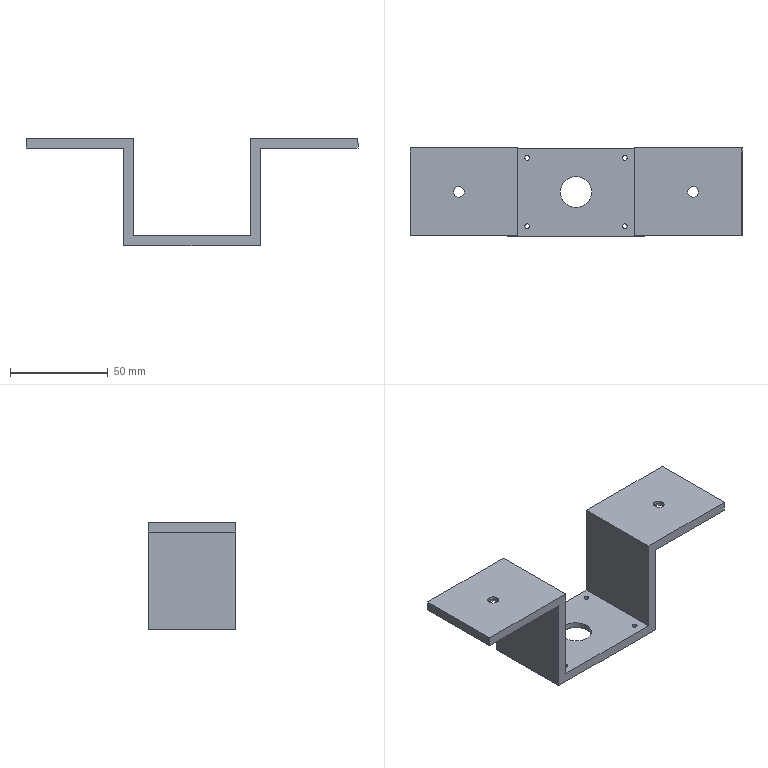Part | SolidWorks | features ICE 2, Cut 1, Extrusion 1, HoleWzd 1 | 1 solid | 41 faces | box 170 x 45 x 55 mm | volume 57748 mm3 | cylinder 20 | plane 17 | cone 4 | commonest cylinder face diameters 2.4 x6 5.5 x4 12.238 x4 2.409 x2 16 x2 30 x2
STEP:
#1=CARTESIAN_POINT('',(61.2,40.,-50.));
#2=VERTEX_POINT('',#1);
#3=CARTESIAN_POINT('',(58.8,40.,-50.));
#4=VERTEX_POINT('',#3);
#5=CARTESIAN_POINT('',(60.,40.,-50.));
#6=DIRECTION('',(0.,0.,-1.));
#7=DIRECTION('',(-1.,0.,0.));
#8=AXIS2_PLACEMENT_3D('',#5,#6,#7);
#9=CIRCLE('',#8,1.2);
#10=EDGE_CURVE('',#2,#4,#9,.T.);
#11=ORIENTED_EDGE('',*,*,#10,.F.);
#12=CARTESIAN_POINT('',(61.2,40.,-55.));
#13=VERTEX_POINT('',#12);
#14=CARTESIAN_POINT('',(61.2,40.,-50.));
#15=DIRECTION('',(0.,0.,-1.));
#16=VECTOR('',#15,1000.);
#17=LINE('',#14,#16);
#18=EDGE_CURVE('',#2,#13,#17,.T.);
#19=ORIENTED_EDGE('',*,*,#18,.T.);
#20=CARTESIAN_POINT('',(58.8,40.,-55.));
#21=VERTEX_POINT('',#20);
#22=CARTESIAN_POINT('',(60.,40.,-55.));
#23=DIRECTION('',(0.,0.,-1.));
#24=DIRECTION('',(-1.,0.,0.));
#25=AXIS2_PLACEMENT_3D('',#22,#23,#24);
#26=CIRCLE('',#25,1.2);
#27=EDGE_CURVE('',#13,#21,#26,.T.);
#28=ORIENTED_EDGE('',*,*,#27,.T.);
#29=CARTESIAN_POINT('',(58.8,40.,-50.));
#30=DIRECTION('',(0.,0.,-1.));
#31=VECTOR('',#30,1000.);
#32=LINE('',#29,#31);
#33=EDGE_CURVE('',#4,#21,#32,.T.);
#34=ORIENTED_EDGE('',*,*,#33,.F.);
#35=EDGE_LOOP('',(#11,#19,#28,#34));
#36=FACE_OUTER_BOUND('',#35,.T.);
#37=CARTESIAN_POINT('',(60.,40.,-50.));
#38=DIRECTION('',(0.,0.,-1.));
#39=DIRECTION('',(-1.,0.,0.));
#40=AXIS2_PLACEMENT_3D('',#37,#38,#39);
#41=CYLINDRICAL_SURFACE('',#40,1.2);
#42=ADVANCED_FACE('',(#36),#41,.F.);
#43=CARTESIAN_POINT('',(111.2,5.,-50.));
#44=VERTEX_POINT('',#43);
#45=CARTESIAN_POINT('',(108.8,5.,-50.));
#46=VERTEX_POINT('',#45);
#47=CARTESIAN_POINT('',(110.,5.,-50.));
#48=DIRECTION('',(0.,0.,-1.));
#49=DIRECTION('',(-1.,0.,0.));
#50=AXIS2_PLACEMENT_3D('',#47,#48,#49);
#51=CIRCLE('',#50,1.2);
#52=EDGE_CURVE('',#44,#46,#51,.T.);
#53=ORIENTED_EDGE('',*,*,#52,.F.);
#54=CARTESIAN_POINT('',(111.2,5.,-55.));
#55=VERTEX_POINT('',#54);
#56=CARTESIAN_POINT('',(111.2,5.,-50.));
#57=DIRECTION('',(0.,0.,-1.));
#58=VECTOR('',#57,1000.);
#59=LINE('',#56,#58);
#60=EDGE_CURVE('',#44,#55,#59,.T.);
#61=ORIENTED_EDGE('',*,*,#60,.T.);
#62=CARTESIAN_POINT('',(108.8,5.,-55.));
#63=VERTEX_POINT('',#62);
#64=CARTESIAN_POINT('',(110.,5.,-55.));
#65=DIRECTION('',(0.,0.,-1.));
#66=DIRECTION('',(-1.,0.,0.));
#67=AXIS2_PLACEMENT_3D('',#64,#65,#66);
#68=CIRCLE('',#67,1.2);
#69=EDGE_CURVE('',#55,#63,#68,.T.);
#70=ORIENTED_EDGE('',*,*,#69,.T.);
#71=CARTESIAN_POINT('',(108.8,5.,-50.));
#72=DIRECTION('',(0.,0.,-1.));
#73=VECTOR('',#72,1000.);
#74=LINE('',#71,#73);
#75=EDGE_CURVE('',#46,#63,#74,.T.);
#76=ORIENTED_EDGE('',*,*,#75,.F.);
#77=EDGE_LOOP('',(#53,#61,#70,#76));
#78=FACE_OUTER_BOUND('',#77,.T.);
#79=CARTESIAN_POINT('',(110.,5.,-50.));
#80=DIRECTION('',(0.,0.,-1.));
#81=DIRECTION('',(-1.,0.,0.));
#82=AXIS2_PLACEMENT_3D('',#79,#80,#81);
#83=CYLINDRICAL_SURFACE('',#82,1.2);
#84=ADVANCED_FACE('',(#78),#83,.F.);
#85=CARTESIAN_POINT('',(111.2,40.,-50.));
#86=VERTEX_POINT('',#85);
#87=CARTESIAN_POINT('',(108.8,40.,-50.));
#88=VERTEX_POINT('',#87);
#89=CARTESIAN_POINT('',(110.,40.,-50.));
#90=DIRECTION('',(0.,0.,-1.));
#91=DIRECTION('',(-1.,0.,0.));
#92=AXIS2_PLACEMENT_3D('',#89,#90,#91);
#93=CIRCLE('',#92,1.2);
#94=EDGE_CURVE('',#86,#88,#93,.T.);
#95=ORIENTED_EDGE('',*,*,#94,.F.);
#96=CARTESIAN_POINT('',(111.2,40.,-55.));
#97=VERTEX_POINT('',#96);
#98=CARTESIAN_POINT('',(111.2,40.,-50.));
#99=DIRECTION('',(0.,0.,-1.));
#100=VECTOR('',#99,1000.);
#101=LINE('',#98,#100);
#102=EDGE_CURVE('',#86,#97,#101,.T.);
#103=ORIENTED_EDGE('',*,*,#102,.T.);
#104=CARTESIAN_POINT('',(108.8,40.,-55.));
#105=VERTEX_POINT('',#104);
#106=CARTESIAN_POINT('',(110.,40.,-55.));
#107=DIRECTION('',(0.,0.,-1.));
#108=DIRECTION('',(-1.,0.,0.));
#109=AXIS2_PLACEMENT_3D('',#106,#107,#108);
#110=CIRCLE('',#109,1.2);
#111=EDGE_CURVE('',#97,#105,#110,.T.);
#112=ORIENTED_EDGE('',*,*,#111,.T.);
#113=CARTESIAN_POINT('',(108.8,40.,-50.));
#114=DIRECTION('',(0.,0.,-1.));
#115=VECTOR('',#114,1000.);
#116=LINE('',#113,#115);
#117=EDGE_CURVE('',#88,#105,#116,.T.);
#118=ORIENTED_EDGE('',*,*,#117,.F.);
#119=EDGE_LOOP('',(#95,#103,#112,#118));
#120=FACE_OUTER_BOUND('',#119,.T.);
#121=CARTESIAN_POINT('',(110.,40.,-50.));
#122=DIRECTION('',(0.,0.,-1.));
#123=DIRECTION('',(-1.,0.,0.));
#124=AXIS2_PLACEMENT_3D('',#121,#122,#123);
#125=CYLINDRICAL_SURFACE('',#124,1.2);
#126=ADVANCED_FACE('',(#120),#125,.F.);
#127=CARTESIAN_POINT('',(61.204,5.,-50.));
#128=VERTEX_POINT('',#127);
#129=CARTESIAN_POINT('',(58.796,5.,-50.));
#130=VERTEX_POINT('',#129);
#131=CARTESIAN_POINT('',(60.,5.,-50.));
#132=DIRECTION('',(0.,0.,-1.));
#133=DIRECTION('',(-1.,0.,0.));
#134=AXIS2_PLACEMENT_3D('',#131,#132,#133);
#135=CIRCLE('',#134,1.204);
#136=EDGE_CURVE('',#128,#130,#135,.T.);
#137=ORIENTED_EDGE('',*,*,#136,.F.);
#138=CARTESIAN_POINT('',(61.204,5.,-55.));
#139=VERTEX_POINT('',#138);
#140=CARTESIAN_POINT('',(61.204,5.,-50.));
#141=DIRECTION('',(0.,0.,-1.));
#142=VECTOR('',#141,1000.);
#143=LINE('',#140,#142);
#144=EDGE_CURVE('',#128,#139,#143,.T.);
#145=ORIENTED_EDGE('',*,*,#144,.T.);
#146=CARTESIAN_POINT('',(58.796,5.,-55.));
#147=VERTEX_POINT('',#146);
#148=CARTESIAN_POINT('',(60.,5.,-55.));
#149=DIRECTION('',(0.,0.,-1.));
#150=DIRECTION('',(-1.,0.,0.));
#151=AXIS2_PLACEMENT_3D('',#148,#149,#150);
#152=CIRCLE('',#151,1.204);
#153=EDGE_CURVE('',#139,#147,#152,.T.);
#154=ORIENTED_EDGE('',*,*,#153,.T.);
#155=CARTESIAN_POINT('',(58.796,5.,-50.));
#156=DIRECTION('',(0.,0.,-1.));
#157=VECTOR('',#156,1000.);
#158=LINE('',#155,#157);
#159=EDGE_CURVE('',#130,#147,#158,.T.);
#160=ORIENTED_EDGE('',*,*,#159,.F.);
#161=EDGE_LOOP('',(#137,#145,#154,#160));
#162=FACE_OUTER_BOUND('',#161,.T.);
#163=CARTESIAN_POINT('',(60.,5.,-50.));
#164=DIRECTION('',(0.,0.,-1.));
#165=DIRECTION('',(-1.,0.,0.));
#166=AXIS2_PLACEMENT_3D('',#163,#164,#165);
#167=CYLINDRICAL_SURFACE('',#166,1.204);
#168=ADVANCED_FACE('',(#162),#167,.F.);
#169=CARTESIAN_POINT('',(100.,22.5,-53.));
#170=VERTEX_POINT('',#169);
#171=CARTESIAN_POINT('',(70.,22.5,-53.));
#172=VERTEX_POINT('',#171);
#173=CARTESIAN_POINT('',(85.,22.5,-53.));
#174=DIRECTION('',(0.,0.,-1.));
#175=DIRECTION('',(-1.,0.,0.));
#176=AXIS2_PLACEMENT_3D('',#173,#174,#175);
#177=CIRCLE('',#176,15.);
#178=EDGE_CURVE('',#170,#172,#177,.T.);
#179=ORIENTED_EDGE('',*,*,#178,.F.);
#180=CARTESIAN_POINT('',(100.,22.5,-55.));
#181=VERTEX_POINT('',#180);
#182=CARTESIAN_POINT('',(100.,22.5,-53.));
#183=DIRECTION('',(0.,0.,-1.));
#184=VECTOR('',#183,1000.);
#185=LINE('',#182,#184);
#186=EDGE_CURVE('',#170,#181,#185,.T.);
#187=ORIENTED_EDGE('',*,*,#186,.T.);
#188=CARTESIAN_POINT('',(70.,22.5,-55.));
#189=VERTEX_POINT('',#188);
#190=CARTESIAN_POINT('',(85.,22.5,-55.));
#191=DIRECTION('',(0.,0.,-1.));
#192=DIRECTION('',(-1.,0.,0.));
#193=AXIS2_PLACEMENT_3D('',#190,#191,#192);
#194=CIRCLE('',#193,15.);
#195=EDGE_CURVE('',#181,#189,#194,.T.);
#196=ORIENTED_EDGE('',*,*,#195,.T.);
#197=CARTESIAN_POINT('',(70.,22.5,-53.));
#198=DIRECTION('',(0.,0.,-1.));
#199=VECTOR('',#198,1000.);
#200=LINE('',#197,#199);
#201=EDGE_CURVE('',#172,#189,#200,.T.);
#202=ORIENTED_EDGE('',*,*,#201,.F.);
#203=EDGE_LOOP('',(#179,#187,#196,#202));
#204=FACE_OUTER_BOUND('',#203,.T.);
#205=CARTESIAN_POINT('',(85.,22.5,-53.));
#206=DIRECTION('',(0.,0.,-1.));
#207=DIRECTION('',(-1.,0.,0.));
#208=AXIS2_PLACEMENT_3D('',#205,#206,#207);
#209=CYLINDRICAL_SURFACE('',#208,15.);
#210=ADVANCED_FACE('',(#204),#209,.F.);
#211=CARTESIAN_POINT('',(151.119,22.5,-4.975));
#212=VERTEX_POINT('',#211);
#213=CARTESIAN_POINT('',(138.881,22.5,-4.975));
#214=VERTEX_POINT('',#213);
#215=CARTESIAN_POINT('',(145.,22.5,-4.975));
#216=DIRECTION('',(0.,0.,-1.));
#217=DIRECTION('',(-1.,0.,0.));
#218=AXIS2_PLACEMENT_3D('',#215,#216,#217);
#219=CIRCLE('',#218,6.119);
#220=EDGE_CURVE('',#212,#214,#219,.T.);
#221=ORIENTED_EDGE('',*,*,#220,.F.);
#222=CARTESIAN_POINT('',(151.144,22.5,-5.));
#223=VERTEX_POINT('',#222);
#224=CARTESIAN_POINT('',(151.144,22.5,-5.));
#225=DIRECTION('',(0.7071,0.,-0.7071));
#226=VECTOR('',#225,1000.);
#227=LINE('',#224,#226);
#228=EDGE_CURVE('',#212,#223,#227,.T.);
#229=ORIENTED_EDGE('',*,*,#228,.T.);
#230=CARTESIAN_POINT('',(138.856,22.5,-5.));
#231=VERTEX_POINT('',#230);
#232=CARTESIAN_POINT('',(145.,22.5,-5.));
#233=DIRECTION('',(0.,0.,-1.));
#234=DIRECTION('',(-1.,0.,0.));
#235=AXIS2_PLACEMENT_3D('',#232,#233,#234);
#236=CIRCLE('',#235,6.144);
#237=EDGE_CURVE('',#223,#231,#236,.T.);
#238=ORIENTED_EDGE('',*,*,#237,.T.);
#239=CARTESIAN_POINT('',(138.856,22.5,-5.));
#240=DIRECTION('',(-0.7071,0.,-0.7071));
#241=VECTOR('',#240,1000.);
#242=LINE('',#239,#241);
#243=EDGE_CURVE('',#214,#231,#242,.T.);
#244=ORIENTED_EDGE('',*,*,#243,.F.);
#245=EDGE_LOOP('',(#221,#229,#238,#244));
#246=FACE_OUTER_BOUND('',#245,.T.);
#247=CARTESIAN_POINT('',(145.,22.5,-5.));
#248=DIRECTION('',(0.,0.,-1.));
#249=DIRECTION('',(-1.,0.,0.));
#250=AXIS2_PLACEMENT_3D('',#247,#248,#249);
#251=CONICAL_SURFACE('',#250,6.144,0.7854);
#252=ADVANCED_FACE('',(#246),#251,.F.);
#253=CARTESIAN_POINT('',(151.119,22.5,-1.5));
#254=VERTEX_POINT('',#253);
#255=CARTESIAN_POINT('',(138.881,22.5,-1.5));
#256=VERTEX_POINT('',#255);
#257=CARTESIAN_POINT('',(145.,22.5,-1.5));
#258=DIRECTION('',(0.,0.,-1.));
#259=DIRECTION('',(-1.,0.,0.));
#260=AXIS2_PLACEMENT_3D('',#257,#258,#259);
#261=CIRCLE('',#260,6.119);
#262=EDGE_CURVE('',#254,#256,#261,.T.);
#263=ORIENTED_EDGE('',*,*,#262,.F.);
#264=CARTESIAN_POINT('',(151.119,22.5,-5.));
#265=DIRECTION('',(0.,0.,-1.));
#266=VECTOR('',#265,1000.);
#267=LINE('',#264,#266);
#268=EDGE_CURVE('',#254,#212,#267,.T.);
#269=ORIENTED_EDGE('',*,*,#268,.T.);
#270=ORIENTED_EDGE('',*,*,#220,.T.);
#271=CARTESIAN_POINT('',(138.881,22.5,-5.));
#272=DIRECTION('',(0.,0.,-1.));
#273=VECTOR('',#272,1000.);
#274=LINE('',#271,#273);
#275=EDGE_CURVE('',#256,#214,#274,.T.);
#276=ORIENTED_EDGE('',*,*,#275,.F.);
#277=EDGE_LOOP('',(#263,#269,#270,#276));
#278=FACE_OUTER_BOUND('',#277,.T.);
#279=CARTESIAN_POINT('',(145.,22.5,-5.));
#280=DIRECTION('',(0.,0.,-1.));
#281=DIRECTION('',(-1.,0.,0.));
#282=AXIS2_PLACEMENT_3D('',#279,#280,#281);
#283=CYLINDRICAL_SURFACE('',#282,6.119);
#284=ADVANCED_FACE('',(#278),#283,.F.);
#285=CARTESIAN_POINT('',(147.75,22.5,0.));
#286=VERTEX_POINT('',#285);
#287=CARTESIAN_POINT('',(142.25,22.5,0.));
#288=VERTEX_POINT('',#287);
#289=CARTESIAN_POINT('',(145.,22.5,0.));
#290=DIRECTION('',(0.,0.,-1.));
#291=DIRECTION('',(-1.,0.,0.));
#292=AXIS2_PLACEMENT_3D('',#289,#290,#291);
#293=CIRCLE('',#292,2.75);
#294=EDGE_CURVE('',#286,#288,#293,.T.);
#295=ORIENTED_EDGE('',*,*,#294,.F.);
#296=CARTESIAN_POINT('',(147.75,22.5,-1.5));
#297=VERTEX_POINT('',#296);
#298=CARTESIAN_POINT('',(147.75,22.5,-5.));
#299=DIRECTION('',(0.,0.,-1.));
#300=VECTOR('',#299,1000.);
#301=LINE('',#298,#300);
#302=EDGE_CURVE('',#286,#297,#301,.T.);
#303=ORIENTED_EDGE('',*,*,#302,.T.);
#304=CARTESIAN_POINT('',(142.25,22.5,-1.5));
#305=VERTEX_POINT('',#304);
#306=CARTESIAN_POINT('',(145.,22.5,-1.5));
#307=DIRECTION('',(0.,0.,-1.));
#308=DIRECTION('',(-1.,0.,0.));
#309=AXIS2_PLACEMENT_3D('',#306,#307,#308);
#310=CIRCLE('',#309,2.75);
#311=EDGE_CURVE('',#297,#305,#310,.T.);
#312=ORIENTED_EDGE('',*,*,#311,.T.);
#313=CARTESIAN_POINT('',(142.25,22.5,-5.));
#314=DIRECTION('',(0.,0.,-1.));
#315=VECTOR('',#314,1000.);
#316=LINE('',#313,#315);
#317=EDGE_CURVE('',#288,#305,#316,.T.);
#318=ORIENTED_EDGE('',*,*,#317,.F.);
#319=EDGE_LOOP('',(#295,#303,#312,#318));
#320=FACE_OUTER_BOUND('',#319,.T.);
#321=CARTESIAN_POINT('',(145.,22.5,-5.));
#322=DIRECTION('',(0.,0.,-1.));
#323=DIRECTION('',(-1.,0.,0.));
#324=AXIS2_PLACEMENT_3D('',#321,#322,#323);
#325=CYLINDRICAL_SURFACE('',#324,2.75);
#326=ADVANCED_FACE('',(#320),#325,.F.);
#327=CARTESIAN_POINT('',(31.119,22.5,-4.975));
#328=VERTEX_POINT('',#327);
#329=CARTESIAN_POINT('',(18.881,22.5,-4.975));
#330=VERTEX_POINT('',#329);
#331=CARTESIAN_POINT('',(25.,22.5,-4.975));
#332=DIRECTION('',(0.,0.,-1.));
#333=DIRECTION('',(-1.,0.,0.));
#334=AXIS2_PLACEMENT_3D('',#331,#332,#333);
#335=CIRCLE('',#334,6.119);
#336=EDGE_CURVE('',#328,#330,#335,.T.);
#337=ORIENTED_EDGE('',*,*,#336,.F.);
#338=CARTESIAN_POINT('',(31.144,22.5,-5.));
#339=VERTEX_POINT('',#338);
#340=CARTESIAN_POINT('',(31.144,22.5,-5.));
#341=DIRECTION('',(0.7071,0.,-0.7071));
#342=VECTOR('',#341,1000.);
#343=LINE('',#340,#342);
#344=EDGE_CURVE('',#328,#339,#343,.T.);
#345=ORIENTED_EDGE('',*,*,#344,.T.);
#346=CARTESIAN_POINT('',(18.856,22.5,-5.));
#347=VERTEX_POINT('',#346);
#348=CARTESIAN_POINT('',(25.,22.5,-5.));
#349=DIRECTION('',(0.,0.,-1.));
#350=DIRECTION('',(-1.,0.,0.));
#351=AXIS2_PLACEMENT_3D('',#348,#349,#350);
#352=CIRCLE('',#351,6.144);
#353=EDGE_CURVE('',#339,#347,#352,.T.);
#354=ORIENTED_EDGE('',*,*,#353,.T.);
#355=CARTESIAN_POINT('',(18.856,22.5,-5.));
#356=DIRECTION('',(-0.7071,0.,-0.7071));
#357=VECTOR('',#356,1000.);
#358=LINE('',#355,#357);
#359=EDGE_CURVE('',#330,#347,#358,.T.);
#360=ORIENTED_EDGE('',*,*,#359,.F.);
#361=EDGE_LOOP('',(#337,#345,#354,#360));
#362=FACE_OUTER_BOUND('',#361,.T.);
#363=CARTESIAN_POINT('',(25.,22.5,-5.));
#364=DIRECTION('',(0.,0.,-1.));
#365=DIRECTION('',(-1.,0.,0.));
#366=AXIS2_PLACEMENT_3D('',#363,#364,#365);
#367=CONICAL_SURFACE('',#366,6.144,0.7854);
#368=ADVANCED_FACE('',(#362),#367,.F.);
#369=CARTESIAN_POINT('',(31.119,22.5,-1.5));
#370=VERTEX_POINT('',#369);
#371=CARTESIAN_POINT('',(18.881,22.5,-1.5));
#372=VERTEX_POINT('',#371);
#373=CARTESIAN_POINT('',(25.,22.5,-1.5));
#374=DIRECTION('',(0.,0.,-1.));
#375=DIRECTION('',(-1.,0.,0.));
#376=AXIS2_PLACEMENT_3D('',#373,#374,#375);
#377=CIRCLE('',#376,6.119);
#378=EDGE_CURVE('',#370,#372,#377,.T.);
#379=ORIENTED_EDGE('',*,*,#378,.F.);
#380=CARTESIAN_POINT('',(31.119,22.5,-5.));
#381=DIRECTION('',(0.,0.,-1.));
#382=VECTOR('',#381,1000.);
#383=LINE('',#380,#382);
#384=EDGE_CURVE('',#370,#328,#383,.T.);
#385=ORIENTED_EDGE('',*,*,#384,.T.);
#386=ORIENTED_EDGE('',*,*,#336,.T.);
#387=CARTESIAN_POINT('',(18.881,22.5,-5.));
#388=DIRECTION('',(0.,0.,-1.));
#389=VECTOR('',#388,1000.);
#390=LINE('',#387,#389);
#391=EDGE_CURVE('',#372,#330,#390,.T.);
#392=ORIENTED_EDGE('',*,*,#391,.F.);
#393=EDGE_LOOP('',(#379,#385,#386,#392));
#394=FACE_OUTER_BOUND('',#393,.T.);
#395=CARTESIAN_POINT('',(25.,22.5,-5.));
#396=DIRECTION('',(0.,0.,-1.));
#397=DIRECTION('',(-1.,0.,0.));
#398=AXIS2_PLACEMENT_3D('',#395,#396,#397);
#399=CYLINDRICAL_SURFACE('',#398,6.119);
#400=ADVANCED_FACE('',(#394),#399,.F.);
#401=CARTESIAN_POINT('',(27.75,22.5,0.));
#402=VERTEX_POINT('',#401);
#403=CARTESIAN_POINT('',(22.25,22.5,0.));
#404=VERTEX_POINT('',#403);
#405=CARTESIAN_POINT('',(25.,22.5,0.));
#406=DIRECTION('',(0.,0.,-1.));
#407=DIRECTION('',(-1.,0.,0.));
#408=AXIS2_PLACEMENT_3D('',#405,#406,#407);
#409=CIRCLE('',#408,2.75);
#410=EDGE_CURVE('',#402,#404,#409,.T.);
#411=ORIENTED_EDGE('',*,*,#410,.F.);
#412=CARTESIAN_POINT('',(27.75,22.5,-1.5));
#413=VERTEX_POINT('',#412);
#414=CARTESIAN_POINT('',(27.75,22.5,-5.));
#415=DIRECTION('',(0.,0.,-1.));
#416=VECTOR('',#415,1000.);
#417=LINE('',#414,#416);
#418=EDGE_CURVE('',#402,#413,#417,.T.);
#419=ORIENTED_EDGE('',*,*,#418,.T.);
#420=CARTESIAN_POINT('',(22.25,22.5,-1.5));
#421=VERTEX_POINT('',#420);
#422=CARTESIAN_POINT('',(25.,22.5,-1.5));
#423=DIRECTION('',(0.,0.,-1.));
#424=DIRECTION('',(-1.,0.,0.));
#425=AXIS2_PLACEMENT_3D('',#422,#423,#424);
#426=CIRCLE('',#425,2.75);
#427=EDGE_CURVE('',#413,#421,#426,.T.);
#428=ORIENTED_EDGE('',*,*,#427,.T.);
#429=CARTESIAN_POINT('',(22.25,22.5,-5.));
#430=DIRECTION('',(0.,0.,-1.));
#431=VECTOR('',#430,1000.);
#432=LINE('',#429,#431);
#433=EDGE_CURVE('',#404,#421,#432,.T.);
#434=ORIENTED_EDGE('',*,*,#433,.F.);
#435=EDGE_LOOP('',(#411,#419,#428,#434));
#436=FACE_OUTER_BOUND('',#435,.T.);
#437=CARTESIAN_POINT('',(25.,22.5,-5.));
#438=DIRECTION('',(0.,0.,-1.));
#439=DIRECTION('',(-1.,0.,0.));
#440=AXIS2_PLACEMENT_3D('',#437,#438,#439);
#441=CYLINDRICAL_SURFACE('',#440,2.75);
#442=ADVANCED_FACE('',(#436),#441,.F.);
#443=CARTESIAN_POINT('',(93.,22.5,-50.));
#444=VERTEX_POINT('',#443);
#445=CARTESIAN_POINT('',(77.,22.5,-50.));
#446=VERTEX_POINT('',#445);
#447=CARTESIAN_POINT('',(85.,22.5,-50.));
#448=DIRECTION('',(0.,0.,-1.));
#449=DIRECTION('',(-1.,0.,0.));
#450=AXIS2_PLACEMENT_3D('',#447,#448,#449);
#451=CIRCLE('',#450,8.);
#452=EDGE_CURVE('',#444,#446,#451,.T.);
#453=ORIENTED_EDGE('',*,*,#452,.F.);
#454=CARTESIAN_POINT('',(93.,22.5,-53.));
#455=VERTEX_POINT('',#454);
#456=CARTESIAN_POINT('',(93.,22.5,-45.));
#457=DIRECTION('',(0.,0.,-1.));
#458=VECTOR('',#457,1000.);
#459=LINE('',#456,#458);
#460=EDGE_CURVE('',#444,#455,#459,.T.);
#461=ORIENTED_EDGE('',*,*,#460,.T.);
#462=CARTESIAN_POINT('',(77.,22.5,-53.));
#463=VERTEX_POINT('',#462);
#464=CARTESIAN_POINT('',(85.,22.5,-53.));
#465=DIRECTION('',(0.,0.,1.));
#466=DIRECTION('',(-1.,0.,0.));
#467=AXIS2_PLACEMENT_3D('',#464,#465,#466);
#468=CIRCLE('',#467,8.);
#469=EDGE_CURVE('',#463,#455,#468,.T.);
#470=ORIENTED_EDGE('',*,*,#469,.F.);
#471=CARTESIAN_POINT('',(77.,22.5,-45.));
#472=DIRECTION('',(0.,0.,-1.));
#473=VECTOR('',#472,1000.);
#474=LINE('',#471,#473);
#475=EDGE_CURVE('',#446,#463,#474,.T.);
#476=ORIENTED_EDGE('',*,*,#475,.F.);
#477=EDGE_LOOP('',(#453,#461,#470,#476));
#478=FACE_OUTER_BOUND('',#477,.T.);
#479=CARTESIAN_POINT('',(85.,22.5,-45.));
#480=DIRECTION('',(0.,0.,-1.));
#481=DIRECTION('',(-1.,0.,0.));
#482=AXIS2_PLACEMENT_3D('',#479,#480,#481);
#483=CYLINDRICAL_SURFACE('',#482,8.);
#484=ADVANCED_FACE('',(#478),#483,.F.);
#485=ORIENTED_EDGE('',*,*,#460,.F.);
#486=CARTESIAN_POINT('',(85.,22.5,-50.));
#487=DIRECTION('',(0.,0.,-1.));
#488=DIRECTION('',(-1.,0.,0.));
#489=AXIS2_PLACEMENT_3D('',#486,#487,#488);
#490=CIRCLE('',#489,8.);
#491=EDGE_CURVE('',#446,#444,#490,.T.);
#492=ORIENTED_EDGE('',*,*,#491,.F.);
#493=ORIENTED_EDGE('',*,*,#475,.T.);
#494=CARTESIAN_POINT('',(85.,22.5,-53.));
#495=DIRECTION('',(0.,0.,1.));
#496=DIRECTION('',(-1.,0.,0.));
#497=AXIS2_PLACEMENT_3D('',#494,#495,#496);
#498=CIRCLE('',#497,8.);
#499=EDGE_CURVE('',#455,#463,#498,.T.);
#500=ORIENTED_EDGE('',*,*,#499,.F.);
#501=EDGE_LOOP('',(#485,#492,#493,#500));
#502=FACE_OUTER_BOUND('',#501,.T.);
#503=CARTESIAN_POINT('',(85.,22.5,-45.));
#504=DIRECTION('',(0.,0.,-1.));
#505=DIRECTION('',(-1.,0.,0.));
#506=AXIS2_PLACEMENT_3D('',#503,#504,#505);
#507=CYLINDRICAL_SURFACE('',#506,8.);
#508=ADVANCED_FACE('',(#502),#507,.F.);
#509=CARTESIAN_POINT('',(0.,0.,-5.));
#510=VERTEX_POINT('',#509);
#511=CARTESIAN_POINT('',(0.,0.,0.));
#512=VERTEX_POINT('',#511);
#513=CARTESIAN_POINT('',(0.,0.,-5.));
#514=DIRECTION('',(0.,0.,1.));
#515=VECTOR('',#514,1000.);
#516=LINE('',#513,#515);
#517=EDGE_CURVE('',#510,#512,#516,.T.);
#518=ORIENTED_EDGE('',*,*,#517,.T.);
#519=CARTESIAN_POINT('',(0.,45.,0.));
#520=VERTEX_POINT('',#519);
#521=CARTESIAN_POINT('',(0.,45.,0.));
#522=DIRECTION('',(0.,-1.,0.));
#523=VECTOR('',#522,1000.);
#524=LINE('',#521,#523);
#525=EDGE_CURVE('',#520,#512,#524,.T.);
#526=ORIENTED_EDGE('',*,*,#525,.F.);
#527=CARTESIAN_POINT('',(0.,45.,-5.));
#528=VERTEX_POINT('',#527);
#529=CARTESIAN_POINT('',(0.,45.,-5.));
#530=DIRECTION('',(0.,0.,1.));
#531=VECTOR('',#530,1000.);
#532=LINE('',#529,#531);
#533=EDGE_CURVE('',#528,#520,#532,.T.);
#534=ORIENTED_EDGE('',*,*,#533,.F.);
#535=CARTESIAN_POINT('',(0.,45.,-5.));
#536=DIRECTION('',(0.,-1.,0.));
#537=VECTOR('',#536,1000.);
#538=LINE('',#535,#537);
#539=EDGE_CURVE('',#528,#510,#538,.T.);
#540=ORIENTED_EDGE('',*,*,#539,.T.);
#541=EDGE_LOOP('',(#518,#526,#534,#540));
#542=FACE_OUTER_BOUND('',#541,.T.);
#543=CARTESIAN_POINT('',(0.,45.,-5.));
#544=DIRECTION('',(1.,0.,0.));
#545=DIRECTION('',(0.,0.,-1.));
#546=AXIS2_PLACEMENT_3D('',#543,#544,#545);
#547=PLANE('',#546);
#548=ADVANCED_FACE('',(#542),#547,.F.);
#549=CARTESIAN_POINT('',(25.,22.5,0.));
#550=DIRECTION('',(0.,0.,-1.));
#551=DIRECTION('',(-1.,0.,0.));
#552=AXIS2_PLACEMENT_3D('',#549,#550,#551);
#553=CIRCLE('',#552,2.75);
#554=EDGE_CURVE('',#404,#402,#553,.T.);
#555=ORIENTED_EDGE('',*,*,#554,.T.);
#556=ORIENTED_EDGE('',*,*,#410,.T.);
#557=EDGE_LOOP('',(#555,#556));
#558=FACE_BOUND('',#557,.T.);
#559=CARTESIAN_POINT('',(55.,0.,0.));
#560=VERTEX_POINT('',#559);
#561=CARTESIAN_POINT('',(0.,0.,0.));
#562=DIRECTION('',(1.,0.,0.));
#563=VECTOR('',#562,1000.);
#564=LINE('',#561,#563);
#565=EDGE_CURVE('',#512,#560,#564,.T.);
#566=ORIENTED_EDGE('',*,*,#565,.T.);
#567=CARTESIAN_POINT('',(55.,45.,0.));
#568=VERTEX_POINT('',#567);
#569=CARTESIAN_POINT('',(55.,45.,0.));
#570=DIRECTION('',(0.,-1.,0.));
#571=VECTOR('',#570,1000.);
#572=LINE('',#569,#571);
#573=EDGE_CURVE('',#568,#560,#572,.T.);
#574=ORIENTED_EDGE('',*,*,#573,.F.);
#575=CARTESIAN_POINT('',(0.,45.,0.));
#576=DIRECTION('',(1.,0.,0.));
#577=VECTOR('',#576,1000.);
#578=LINE('',#575,#577);
#579=EDGE_CURVE('',#520,#568,#578,.T.);
#580=ORIENTED_EDGE('',*,*,#579,.F.);
#581=ORIENTED_EDGE('',*,*,#525,.T.);
#582=EDGE_LOOP('',(#566,#574,#580,#581));
#583=FACE_OUTER_BOUND('',#582,.T.);
#584=CARTESIAN_POINT('',(0.,45.,0.));
#585=DIRECTION('',(0.,0.,-1.));
#586=DIRECTION('',(-1.,0.,0.));
#587=AXIS2_PLACEMENT_3D('',#584,#585,#586);
#588=PLANE('',#587);
#589=ADVANCED_FACE('',(#558,#583),#588,.F.);
#590=CARTESIAN_POINT('',(55.,0.,-50.));
#591=VERTEX_POINT('',#590);
#592=CARTESIAN_POINT('',(55.,0.,0.));
#593=DIRECTION('',(0.,0.,-1.));
#594=VECTOR('',#593,1000.);
#595=LINE('',#592,#594);
#596=EDGE_CURVE('',#560,#591,#595,.T.);
#597=ORIENTED_EDGE('',*,*,#596,.T.);
#598=CARTESIAN_POINT('',(55.,45.,-50.));
#599=VERTEX_POINT('',#598);
#600=CARTESIAN_POINT('',(55.,45.,-50.));
#601=DIRECTION('',(0.,-1.,0.));
#602=VECTOR('',#601,1000.);
#603=LINE('',#600,#602);
#604=EDGE_CURVE('',#599,#591,#603,.T.);
#605=ORIENTED_EDGE('',*,*,#604,.F.);
#606=CARTESIAN_POINT('',(55.,45.,0.));
#607=DIRECTION('',(0.,0.,-1.));
#608=VECTOR('',#607,1000.);
#609=LINE('',#606,#608);
#610=EDGE_CURVE('',#568,#599,#609,.T.);
#611=ORIENTED_EDGE('',*,*,#610,.F.);
#612=ORIENTED_EDGE('',*,*,#573,.T.);
#613=EDGE_LOOP('',(#597,#605,#611,#612));
#614=FACE_OUTER_BOUND('',#613,.T.);
#615=CARTESIAN_POINT('',(55.,45.,0.));
#616=DIRECTION('',(-1.,0.,0.));
#617=DIRECTION('',(0.,0.,1.));
#618=AXIS2_PLACEMENT_3D('',#615,#616,#617);
#619=PLANE('',#618);
#620=ADVANCED_FACE('',(#614),#619,.F.);
#621=CARTESIAN_POINT('',(60.,40.,-50.));
#622=DIRECTION('',(0.,0.,-1.));
#623=DIRECTION('',(-1.,0.,0.));
#624=AXIS2_PLACEMENT_3D('',#621,#622,#623);
#625=CIRCLE('',#624,1.2);
#626=EDGE_CURVE('',#4,#2,#625,.T.);
#627=ORIENTED_EDGE('',*,*,#626,.T.);
#628=ORIENTED_EDGE('',*,*,#10,.T.);
#629=EDGE_LOOP('',(#627,#628));
#630=FACE_BOUND('',#629,.T.);
#631=CARTESIAN_POINT('',(110.,5.,-50.));
#632=DIRECTION('',(0.,0.,-1.));
#633=DIRECTION('',(-1.,0.,0.));
#634=AXIS2_PLACEMENT_3D('',#631,#632,#633);
#635=CIRCLE('',#634,1.2);
#636=EDGE_CURVE('',#46,#44,#635,.T.);
#637=ORIENTED_EDGE('',*,*,#636,.T.);
#638=ORIENTED_EDGE('',*,*,#52,.T.);
#639=EDGE_LOOP('',(#637,#638));
#640=FACE_BOUND('',#639,.T.);
#641=CARTESIAN_POINT('',(110.,40.,-50.));
#642=DIRECTION('',(0.,0.,-1.));
#643=DIRECTION('',(-1.,0.,0.));
#644=AXIS2_PLACEMENT_3D('',#641,#642,#643);
#645=CIRCLE('',#644,1.2);
#646=EDGE_CURVE('',#88,#86,#645,.T.);
#647=ORIENTED_EDGE('',*,*,#646,.T.);
#648=ORIENTED_EDGE('',*,*,#94,.T.);
#649=EDGE_LOOP('',(#647,#648));
#650=FACE_BOUND('',#649,.T.);
#651=CARTESIAN_POINT('',(60.,5.,-50.));
#652=DIRECTION('',(0.,0.,-1.));
#653=DIRECTION('',(-1.,0.,0.));
#654=AXIS2_PLACEMENT_3D('',#651,#652,#653);
#655=CIRCLE('',#654,1.204);
#656=EDGE_CURVE('',#130,#128,#655,.T.);
#657=ORIENTED_EDGE('',*,*,#656,.T.);
#658=ORIENTED_EDGE('',*,*,#136,.T.);
#659=EDGE_LOOP('',(#657,#658));
#660=FACE_BOUND('',#659,.T.);
#661=ORIENTED_EDGE('',*,*,#491,.T.);
#662=ORIENTED_EDGE('',*,*,#452,.T.);
#663=EDGE_LOOP('',(#661,#662));
#664=FACE_BOUND('',#663,.T.);
#665=CARTESIAN_POINT('',(115.,0.,-50.));
#666=VERTEX_POINT('',#665);
#667=CARTESIAN_POINT('',(55.,0.,-50.));
#668=DIRECTION('',(1.,0.,0.));
#669=VECTOR('',#668,1000.);
#670=LINE('',#667,#669);
#671=EDGE_CURVE('',#591,#666,#670,.T.);
#672=ORIENTED_EDGE('',*,*,#671,.T.);
#673=CARTESIAN_POINT('',(115.,45.,-50.));
#674=VERTEX_POINT('',#673);
#675=CARTESIAN_POINT('',(115.,45.,-50.));
#676=DIRECTION('',(0.,-1.,0.));
#677=VECTOR('',#676,1000.);
#678=LINE('',#675,#677);
#679=EDGE_CURVE('',#674,#666,#678,.T.);
#680=ORIENTED_EDGE('',*,*,#679,.F.);
#681=CARTESIAN_POINT('',(55.,45.,-50.));
#682=DIRECTION('',(1.,0.,0.));
#683=VECTOR('',#682,1000.);
#684=LINE('',#681,#683);
#685=EDGE_CURVE('',#599,#674,#684,.T.);
#686=ORIENTED_EDGE('',*,*,#685,.F.);
#687=ORIENTED_EDGE('',*,*,#604,.T.);
#688=EDGE_LOOP('',(#672,#680,#686,#687));
#689=FACE_OUTER_BOUND('',#688,.T.);
#690=CARTESIAN_POINT('',(55.,45.,-50.));
#691=DIRECTION('',(0.,0.,-1.));
#692=DIRECTION('',(-1.,0.,0.));
#693=AXIS2_PLACEMENT_3D('',#690,#691,#692);
#694=PLANE('',#693);
#695=ADVANCED_FACE('',(#630,#640,#650,#660,#664,#689),#694,.F.);
#696=CARTESIAN_POINT('',(115.,0.,0.));
#697=VERTEX_POINT('',#696);
#698=CARTESIAN_POINT('',(115.,0.,-50.));
#699=DIRECTION('',(0.,0.,1.));
#700=VECTOR('',#699,1000.);
#701=LINE('',#698,#700);
#702=EDGE_CURVE('',#666,#697,#701,.T.);
#703=ORIENTED_EDGE('',*,*,#702,.T.);
#704=CARTESIAN_POINT('',(115.,45.,0.));
#705=VERTEX_POINT('',#704);
#706=CARTESIAN_POINT('',(115.,45.,0.));
#707=DIRECTION('',(0.,-1.,0.));
#708=VECTOR('',#707,1000.);
#709=LINE('',#706,#708);
#710=EDGE_CURVE('',#705,#697,#709,.T.);
#711=ORIENTED_EDGE('',*,*,#710,.F.);
#712=CARTESIAN_POINT('',(115.,45.,-50.));
#713=DIRECTION('',(0.,0.,1.));
#714=VECTOR('',#713,1000.);
#715=LINE('',#712,#714);
#716=EDGE_CURVE('',#674,#705,#715,.T.);
#717=ORIENTED_EDGE('',*,*,#716,.F.);
#718=ORIENTED_EDGE('',*,*,#679,.T.);
#719=EDGE_LOOP('',(#703,#711,#717,#718));
#720=FACE_OUTER_BOUND('',#719,.T.);
#721=CARTESIAN_POINT('',(115.,45.,-50.));
#722=DIRECTION('',(1.,0.,0.));
#723=DIRECTION('',(0.,0.,-1.));
#724=AXIS2_PLACEMENT_3D('',#721,#722,#723);
#725=PLANE('',#724);
#726=ADVANCED_FACE('',(#720),#725,.F.);
#727=CARTESIAN_POINT('',(145.,22.5,0.));
#728=DIRECTION('',(0.,0.,-1.));
#729=DIRECTION('',(-1.,0.,0.));
#730=AXIS2_PLACEMENT_3D('',#727,#728,#729);
#731=CIRCLE('',#730,2.75);
#732=EDGE_CURVE('',#288,#286,#731,.T.);
#733=ORIENTED_EDGE('',*,*,#732,.T.);
#734=ORIENTED_EDGE('',*,*,#294,.T.);
#735=EDGE_LOOP('',(#733,#734));
#736=FACE_BOUND('',#735,.T.);
#737=CARTESIAN_POINT('',(170.,0.,0.));
#738=VERTEX_POINT('',#737);
#739=CARTESIAN_POINT('',(115.,0.,0.));
#740=DIRECTION('',(1.,0.,0.));
#741=VECTOR('',#740,1000.);
#742=LINE('',#739,#741);
#743=EDGE_CURVE('',#697,#738,#742,.T.);
#744=ORIENTED_EDGE('',*,*,#743,.T.);
#745=CARTESIAN_POINT('',(170.,45.,0.));
#746=VERTEX_POINT('',#745);
#747=CARTESIAN_POINT('',(170.,45.,0.));
#748=DIRECTION('',(0.,-1.,0.));
#749=VECTOR('',#748,1000.);
#750=LINE('',#747,#749);
#751=EDGE_CURVE('',#746,#738,#750,.T.);
#752=ORIENTED_EDGE('',*,*,#751,.F.);
#753=CARTESIAN_POINT('',(115.,45.,0.));
#754=DIRECTION('',(1.,0.,0.));
#755=VECTOR('',#754,1000.);
#756=LINE('',#753,#755);
#757=EDGE_CURVE('',#705,#746,#756,.T.);
#758=ORIENTED_EDGE('',*,*,#757,.F.);
#759=ORIENTED_EDGE('',*,*,#710,.T.);
#760=EDGE_LOOP('',(#744,#752,#758,#759));
#761=FACE_OUTER_BOUND('',#760,.T.);
#762=CARTESIAN_POINT('',(115.,45.,0.));
#763=DIRECTION('',(0.,0.,-1.));
#764=DIRECTION('',(-1.,0.,0.));
#765=AXIS2_PLACEMENT_3D('',#762,#763,#764);
#766=PLANE('',#765);
#767=ADVANCED_FACE('',(#736,#761),#766,.F.);
#768=CARTESIAN_POINT('',(170.,0.,-5.));
#769=VERTEX_POINT('',#768);
#770=CARTESIAN_POINT('',(170.,0.,0.));
#771=DIRECTION('',(0.,0.,-1.));
#772=VECTOR('',#771,1000.);
#773=LINE('',#770,#772);
#774=EDGE_CURVE('',#738,#769,#773,.T.);
#775=ORIENTED_EDGE('',*,*,#774,.T.);
#776=CARTESIAN_POINT('',(170.,45.,-5.));
#777=VERTEX_POINT('',#776);
#778=CARTESIAN_POINT('',(170.,45.,-5.));
#779=DIRECTION('',(0.,-1.,0.));
#780=VECTOR('',#779,1000.);
#781=LINE('',#778,#780);
#782=EDGE_CURVE('',#777,#769,#781,.T.);
#783=ORIENTED_EDGE('',*,*,#782,.F.);
#784=CARTESIAN_POINT('',(170.,45.,0.));
#785=DIRECTION('',(0.,0.,-1.));
#786=VECTOR('',#785,1000.);
#787=LINE('',#784,#786);
#788=EDGE_CURVE('',#746,#777,#787,.T.);
#789=ORIENTED_EDGE('',*,*,#788,.F.);
#790=ORIENTED_EDGE('',*,*,#751,.T.);
#791=EDGE_LOOP('',(#775,#783,#789,#790));
#792=FACE_OUTER_BOUND('',#791,.T.);
#793=CARTESIAN_POINT('',(170.,45.,0.));
#794=DIRECTION('',(-1.,0.,0.));
#795=DIRECTION('',(0.,0.,1.));
#796=AXIS2_PLACEMENT_3D('',#793,#794,#795);
#797=PLANE('',#796);
#798=ADVANCED_FACE('',(#792),#797,.F.);
#799=CARTESIAN_POINT('',(145.,22.5,-5.));
#800=DIRECTION('',(0.,0.,-1.));
#801=DIRECTION('',(-1.,0.,0.));
#802=AXIS2_PLACEMENT_3D('',#799,#800,#801);
#803=CIRCLE('',#802,6.144);
#804=EDGE_CURVE('',#231,#223,#803,.T.);
#805=ORIENTED_EDGE('',*,*,#804,.F.);
#806=ORIENTED_EDGE('',*,*,#237,.F.);
#807=EDGE_LOOP('',(#805,#806));
#808=FACE_BOUND('',#807,.T.);
#809=CARTESIAN_POINT('',(120.,0.,-5.));
#810=VERTEX_POINT('',#809);
#811=CARTESIAN_POINT('',(170.,0.,-5.));
#812=DIRECTION('',(-1.,0.,0.));
#813=VECTOR('',#812,1000.);
#814=LINE('',#811,#813);
#815=EDGE_CURVE('',#769,#810,#814,.T.);
#816=ORIENTED_EDGE('',*,*,#815,.T.);
#817=CARTESIAN_POINT('',(120.,45.,-5.));
#818=VERTEX_POINT('',#817);
#819=CARTESIAN_POINT('',(120.,45.,-5.));
#820=DIRECTION('',(0.,-1.,0.));
#821=VECTOR('',#820,1000.);
#822=LINE('',#819,#821);
#823=EDGE_CURVE('',#818,#810,#822,.T.);
#824=ORIENTED_EDGE('',*,*,#823,.F.);
#825=CARTESIAN_POINT('',(170.,45.,-5.));
#826=DIRECTION('',(-1.,0.,0.));
#827=VECTOR('',#826,1000.);
#828=LINE('',#825,#827);
#829=EDGE_CURVE('',#777,#818,#828,.T.);
#830=ORIENTED_EDGE('',*,*,#829,.F.);
#831=ORIENTED_EDGE('',*,*,#782,.T.);
#832=EDGE_LOOP('',(#816,#824,#830,#831));
#833=FACE_OUTER_BOUND('',#832,.T.);
#834=CARTESIAN_POINT('',(170.,45.,-5.));
#835=DIRECTION('',(0.,0.,1.));
#836=DIRECTION('',(1.,0.,0.));
#837=AXIS2_PLACEMENT_3D('',#834,#835,#836);
#838=PLANE('',#837);
#839=ADVANCED_FACE('',(#808,#833),#838,.F.);
#840=CARTESIAN_POINT('',(120.,0.,-55.));
#841=VERTEX_POINT('',#840);
#842=CARTESIAN_POINT('',(120.,0.,-5.));
#843=DIRECTION('',(0.,0.,-1.));
#844=VECTOR('',#843,1000.);
#845=LINE('',#842,#844);
#846=EDGE_CURVE('',#810,#841,#845,.T.);
#847=ORIENTED_EDGE('',*,*,#846,.T.);
#848=CARTESIAN_POINT('',(120.,45.,-55.));
#849=VERTEX_POINT('',#848);
#850=CARTESIAN_POINT('',(120.,45.,-55.));
#851=DIRECTION('',(0.,-1.,0.));
#852=VECTOR('',#851,1000.);
#853=LINE('',#850,#852);
#854=EDGE_CURVE('',#849,#841,#853,.T.);
#855=ORIENTED_EDGE('',*,*,#854,.F.);
#856=CARTESIAN_POINT('',(120.,45.,-5.));
#857=DIRECTION('',(0.,0.,-1.));
#858=VECTOR('',#857,1000.);
#859=LINE('',#856,#858);
#860=EDGE_CURVE('',#818,#849,#859,.T.);
#861=ORIENTED_EDGE('',*,*,#860,.F.);
#862=ORIENTED_EDGE('',*,*,#823,.T.);
#863=EDGE_LOOP('',(#847,#855,#861,#862));
#864=FACE_OUTER_BOUND('',#863,.T.);
#865=CARTESIAN_POINT('',(120.,45.,-5.));
#866=DIRECTION('',(-1.,0.,0.));
#867=DIRECTION('',(0.,0.,1.));
#868=AXIS2_PLACEMENT_3D('',#865,#866,#867);
#869=PLANE('',#868);
#870=ADVANCED_FACE('',(#864),#869,.F.);
#871=CARTESIAN_POINT('',(60.,40.,-55.));
#872=DIRECTION('',(0.,0.,-1.));
#873=DIRECTION('',(-1.,0.,0.));
#874=AXIS2_PLACEMENT_3D('',#871,#872,#873);
#875=CIRCLE('',#874,1.2);
#876=EDGE_CURVE('',#21,#13,#875,.T.);
#877=ORIENTED_EDGE('',*,*,#876,.F.);
#878=ORIENTED_EDGE('',*,*,#27,.F.);
#879=EDGE_LOOP('',(#877,#878));
#880=FACE_BOUND('',#879,.T.);
#881=CARTESIAN_POINT('',(110.,5.,-55.));
#882=DIRECTION('',(0.,0.,-1.));
#883=DIRECTION('',(-1.,0.,0.));
#884=AXIS2_PLACEMENT_3D('',#881,#882,#883);
#885=CIRCLE('',#884,1.2);
#886=EDGE_CURVE('',#63,#55,#885,.T.);
#887=ORIENTED_EDGE('',*,*,#886,.F.);
#888=ORIENTED_EDGE('',*,*,#69,.F.);
#889=EDGE_LOOP('',(#887,#888));
#890=FACE_BOUND('',#889,.T.);
#891=CARTESIAN_POINT('',(110.,40.,-55.));
#892=DIRECTION('',(0.,0.,-1.));
#893=DIRECTION('',(-1.,0.,0.));
#894=AXIS2_PLACEMENT_3D('',#891,#892,#893);
#895=CIRCLE('',#894,1.2);
#896=EDGE_CURVE('',#105,#97,#895,.T.);
#897=ORIENTED_EDGE('',*,*,#896,.F.);
#898=ORIENTED_EDGE('',*,*,#111,.F.);
#899=EDGE_LOOP('',(#897,#898));
#900=FACE_BOUND('',#899,.T.);
#901=CARTESIAN_POINT('',(60.,5.,-55.));
#902=DIRECTION('',(0.,0.,-1.));
#903=DIRECTION('',(-1.,0.,0.));
#904=AXIS2_PLACEMENT_3D('',#901,#902,#903);
#905=CIRCLE('',#904,1.204);
#906=EDGE_CURVE('',#147,#139,#905,.T.);
#907=ORIENTED_EDGE('',*,*,#906,.F.);
#908=ORIENTED_EDGE('',*,*,#153,.F.);
#909=EDGE_LOOP('',(#907,#908));
#910=FACE_BOUND('',#909,.T.);
#911=CARTESIAN_POINT('',(85.,22.5,-55.));
#912=DIRECTION('',(0.,0.,-1.));
#913=DIRECTION('',(-1.,0.,0.));
#914=AXIS2_PLACEMENT_3D('',#911,#912,#913);
#915=CIRCLE('',#914,15.);
#916=EDGE_CURVE('',#189,#181,#915,.T.);
#917=ORIENTED_EDGE('',*,*,#916,.F.);
#918=ORIENTED_EDGE('',*,*,#195,.F.);
#919=EDGE_LOOP('',(#917,#918));
#920=FACE_BOUND('',#919,.T.);
#921=CARTESIAN_POINT('',(50.,0.,-55.));
#922=VERTEX_POINT('',#921);
#923=CARTESIAN_POINT('',(120.,0.,-55.));
#924=DIRECTION('',(-1.,0.,0.));
#925=VECTOR('',#924,1000.);
#926=LINE('',#923,#925);
#927=EDGE_CURVE('',#841,#922,#926,.T.);
#928=ORIENTED_EDGE('',*,*,#927,.T.);
#929=CARTESIAN_POINT('',(50.,45.,-55.));
#930=VERTEX_POINT('',#929);
#931=CARTESIAN_POINT('',(50.,45.,-55.));
#932=DIRECTION('',(0.,-1.,0.));
#933=VECTOR('',#932,1000.);
#934=LINE('',#931,#933);
#935=EDGE_CURVE('',#930,#922,#934,.T.);
#936=ORIENTED_EDGE('',*,*,#935,.F.);
#937=CARTESIAN_POINT('',(120.,45.,-55.));
#938=DIRECTION('',(-1.,0.,0.));
#939=VECTOR('',#938,1000.);
#940=LINE('',#937,#939);
#941=EDGE_CURVE('',#849,#930,#940,.T.);
#942=ORIENTED_EDGE('',*,*,#941,.F.);
#943=ORIENTED_EDGE('',*,*,#854,.T.);
#944=EDGE_LOOP('',(#928,#936,#942,#943));
#945=FACE_OUTER_BOUND('',#944,.T.);
#946=CARTESIAN_POINT('',(120.,45.,-55.));
#947=DIRECTION('',(0.,0.,1.));
#948=DIRECTION('',(1.,0.,0.));
#949=AXIS2_PLACEMENT_3D('',#946,#947,#948);
#950=PLANE('',#949);
#951=ADVANCED_FACE('',(#880,#890,#900,#910,#920,#945),#950,.F.);
#952=CARTESIAN_POINT('',(50.,0.,-5.));
#953=VERTEX_POINT('',#952);
#954=CARTESIAN_POINT('',(50.,0.,-55.));
#955=DIRECTION('',(0.,0.,1.));
#956=VECTOR('',#955,1000.);
#957=LINE('',#954,#956);
#958=EDGE_CURVE('',#922,#953,#957,.T.);
#959=ORIENTED_EDGE('',*,*,#958,.T.);
#960=CARTESIAN_POINT('',(50.,45.,-5.));
#961=VERTEX_POINT('',#960);
#962=CARTESIAN_POINT('',(50.,45.,-5.));
#963=DIRECTION('',(0.,-1.,0.));
#964=VECTOR('',#963,1000.);
#965=LINE('',#962,#964);
#966=EDGE_CURVE('',#961,#953,#965,.T.);
#967=ORIENTED_EDGE('',*,*,#966,.F.);
#968=CARTESIAN_POINT('',(50.,45.,-55.));
#969=DIRECTION('',(0.,0.,1.));
#970=VECTOR('',#969,1000.);
#971=LINE('',#968,#970);
#972=EDGE_CURVE('',#930,#961,#971,.T.);
#973=ORIENTED_EDGE('',*,*,#972,.F.);
#974=ORIENTED_EDGE('',*,*,#935,.T.);
#975=EDGE_LOOP('',(#959,#967,#973,#974));
#976=FACE_OUTER_BOUND('',#975,.T.);
#977=CARTESIAN_POINT('',(50.,45.,-55.));
#978=DIRECTION('',(1.,0.,0.));
#979=DIRECTION('',(0.,0.,-1.));
#980=AXIS2_PLACEMENT_3D('',#977,#978,#979);
#981=PLANE('',#980);
#982=ADVANCED_FACE('',(#976),#981,.F.);
#983=CARTESIAN_POINT('',(25.,22.5,-5.));
#984=DIRECTION('',(0.,0.,-1.));
#985=DIRECTION('',(-1.,0.,0.));
#986=AXIS2_PLACEMENT_3D('',#983,#984,#985);
#987=CIRCLE('',#986,6.144);
#988=EDGE_CURVE('',#347,#339,#987,.T.);
#989=ORIENTED_EDGE('',*,*,#988,.F.);
#990=ORIENTED_EDGE('',*,*,#353,.F.);
#991=EDGE_LOOP('',(#989,#990));
#992=FACE_BOUND('',#991,.T.);
#993=CARTESIAN_POINT('',(50.,0.,-5.));
#994=DIRECTION('',(-1.,0.,0.));
#995=VECTOR('',#994,1000.);
#996=LINE('',#993,#995);
#997=EDGE_CURVE('',#953,#510,#996,.T.);
#998=ORIENTED_EDGE('',*,*,#997,.T.);
#999=ORIENTED_EDGE('',*,*,#539,.F.);
#1000=CARTESIAN_POINT('',(50.,45.,-5.));
#1001=DIRECTION('',(-1.,0.,0.));
#1002=VECTOR('',#1001,1000.);
#1003=LINE('',#1000,#1002);
#1004=EDGE_CURVE('',#961,#528,#1003,.T.);
#1005=ORIENTED_EDGE('',*,*,#1004,.F.);
#1006=ORIENTED_EDGE('',*,*,#966,.T.);
#1007=EDGE_LOOP('',(#998,#999,#1005,#1006));
#1008=FACE_OUTER_BOUND('',#1007,.T.);
#1009=CARTESIAN_POINT('',(50.,45.,-5.));
#1010=DIRECTION('',(0.,0.,1.));
#1011=DIRECTION('',(1.,0.,0.));
#1012=AXIS2_PLACEMENT_3D('',#1009,#1010,#1011);
#1013=PLANE('',#1012);
#1014=ADVANCED_FACE('',(#992,#1008),#1013,.F.);
#1015=ORIENTED_EDGE('',*,*,#533,.T.);
#1016=ORIENTED_EDGE('',*,*,#579,.T.);
#1017=ORIENTED_EDGE('',*,*,#610,.T.);
#1018=ORIENTED_EDGE('',*,*,#685,.T.);
#1019=ORIENTED_EDGE('',*,*,#716,.T.);
#1020=ORIENTED_EDGE('',*,*,#757,.T.);
#1021=ORIENTED_EDGE('',*,*,#788,.T.);
#1022=ORIENTED_EDGE('',*,*,#829,.T.);
#1023=ORIENTED_EDGE('',*,*,#860,.T.);
#1024=ORIENTED_EDGE('',*,*,#941,.T.);
#1025=ORIENTED_EDGE('',*,*,#972,.T.);
#1026=ORIENTED_EDGE('',*,*,#1004,.T.);
#1027=EDGE_LOOP('',(#1015,#1016,#1017,#1018,#1019,#1020,#1021,#1022,#1023,#1024,#1025,#1026));
#1028=FACE_OUTER_BOUND('',#1027,.T.);
#1029=CARTESIAN_POINT('',(0.,45.,0.));
#1030=DIRECTION('',(0.,1.,0.));
#1031=DIRECTION('',(0.,0.,1.));
#1032=AXIS2_PLACEMENT_3D('',#1029,#1030,#1031);
#1033=PLANE('',#1032);
#1034=ADVANCED_FACE('',(#1028),#1033,.T.);
#1035=ORIENTED_EDGE('',*,*,#517,.F.);
#1036=ORIENTED_EDGE('',*,*,#997,.F.);
#1037=ORIENTED_EDGE('',*,*,#958,.F.);
#1038=ORIENTED_EDGE('',*,*,#927,.F.);
#1039=ORIENTED_EDGE('',*,*,#846,.F.);
#1040=ORIENTED_EDGE('',*,*,#815,.F.);
#1041=ORIENTED_EDGE('',*,*,#774,.F.);
#1042=ORIENTED_EDGE('',*,*,#743,.F.);
#1043=ORIENTED_EDGE('',*,*,#702,.F.);
#1044=ORIENTED_EDGE('',*,*,#671,.F.);
#1045=ORIENTED_EDGE('',*,*,#596,.F.);
#1046=ORIENTED_EDGE('',*,*,#565,.F.);
#1047=EDGE_LOOP('',(#1035,#1036,#1037,#1038,#1039,#1040,#1041,#1042,#1043,#1044,#1045,#1046));
#1048=FACE_OUTER_BOUND('',#1047,.T.);
#1049=CARTESIAN_POINT('',(0.,0.,0.));
#1050=DIRECTION('',(0.,1.,0.));
#1051=DIRECTION('',(0.,0.,1.));
#1052=AXIS2_PLACEMENT_3D('',#1049,#1050,#1051);
#1053=PLANE('',#1052);
#1054=ADVANCED_FACE('',(#1048),#1053,.F.);
#1055=ORIENTED_EDGE('',*,*,#418,.F.);
#1056=ORIENTED_EDGE('',*,*,#554,.F.);
#1057=ORIENTED_EDGE('',*,*,#433,.T.);
#1058=CARTESIAN_POINT('',(25.,22.5,-1.5));
#1059=DIRECTION('',(0.,0.,-1.));
#1060=DIRECTION('',(-1.,0.,0.));
#1061=AXIS2_PLACEMENT_3D('',#1058,#1059,#1060);
#1062=CIRCLE('',#1061,2.75);
#1063=EDGE_CURVE('',#421,#413,#1062,.T.);
#1064=ORIENTED_EDGE('',*,*,#1063,.T.);
#1065=EDGE_LOOP('',(#1055,#1056,#1057,#1064));
#1066=FACE_OUTER_BOUND('',#1065,.T.);
#1067=CARTESIAN_POINT('',(25.,22.5,-5.));
#1068=DIRECTION('',(0.,0.,-1.));
#1069=DIRECTION('',(-1.,0.,0.));
#1070=AXIS2_PLACEMENT_3D('',#1067,#1068,#1069);
#1071=CYLINDRICAL_SURFACE('',#1070,2.75);
#1072=ADVANCED_FACE('',(#1066),#1071,.F.);
#1073=ORIENTED_EDGE('',*,*,#1063,.F.);
#1074=ORIENTED_EDGE('',*,*,#427,.F.);
#1075=EDGE_LOOP('',(#1073,#1074));
#1076=FACE_BOUND('',#1075,.T.);
#1077=CARTESIAN_POINT('',(25.,22.5,-1.5));
#1078=DIRECTION('',(0.,0.,-1.));
#1079=DIRECTION('',(-1.,0.,0.));
#1080=AXIS2_PLACEMENT_3D('',#1077,#1078,#1079);
#1081=CIRCLE('',#1080,6.119);
#1082=EDGE_CURVE('',#372,#370,#1081,.T.);
#1083=ORIENTED_EDGE('',*,*,#1082,.T.);
#1084=ORIENTED_EDGE('',*,*,#378,.T.);
#1085=EDGE_LOOP('',(#1083,#1084));
#1086=FACE_OUTER_BOUND('',#1085,.T.);
#1087=CARTESIAN_POINT('',(31.119,22.5,-1.5));
#1088=DIRECTION('',(0.,0.,1.));
#1089=DIRECTION('',(1.,0.,0.));
#1090=AXIS2_PLACEMENT_3D('',#1087,#1088,#1089);
#1091=PLANE('',#1090);
#1092=ADVANCED_FACE('',(#1076,#1086),#1091,.F.);
#1093=ORIENTED_EDGE('',*,*,#384,.F.);
#1094=ORIENTED_EDGE('',*,*,#1082,.F.);
#1095=ORIENTED_EDGE('',*,*,#391,.T.);
#1096=CARTESIAN_POINT('',(25.,22.5,-4.975));
#1097=DIRECTION('',(0.,0.,-1.));
#1098=DIRECTION('',(-1.,0.,0.));
#1099=AXIS2_PLACEMENT_3D('',#1096,#1097,#1098);
#1100=CIRCLE('',#1099,6.119);
#1101=EDGE_CURVE('',#330,#328,#1100,.T.);
#1102=ORIENTED_EDGE('',*,*,#1101,.T.);
#1103=EDGE_LOOP('',(#1093,#1094,#1095,#1102));
#1104=FACE_OUTER_BOUND('',#1103,.T.);
#1105=CARTESIAN_POINT('',(25.,22.5,-5.));
#1106=DIRECTION('',(0.,0.,-1.));
#1107=DIRECTION('',(-1.,0.,0.));
#1108=AXIS2_PLACEMENT_3D('',#1105,#1106,#1107);
#1109=CYLINDRICAL_SURFACE('',#1108,6.119);
#1110=ADVANCED_FACE('',(#1104),#1109,.F.);
#1111=ORIENTED_EDGE('',*,*,#344,.F.);
#1112=ORIENTED_EDGE('',*,*,#1101,.F.);
#1113=ORIENTED_EDGE('',*,*,#359,.T.);
#1114=ORIENTED_EDGE('',*,*,#988,.T.);
#1115=EDGE_LOOP('',(#1111,#1112,#1113,#1114));
#1116=FACE_OUTER_BOUND('',#1115,.T.);
#1117=CARTESIAN_POINT('',(25.,22.5,-5.));
#1118=DIRECTION('',(0.,0.,-1.));
#1119=DIRECTION('',(-1.,0.,0.));
#1120=AXIS2_PLACEMENT_3D('',#1117,#1118,#1119);
#1121=CONICAL_SURFACE('',#1120,6.144,0.7854);
#1122=ADVANCED_FACE('',(#1116),#1121,.F.);
#1123=ORIENTED_EDGE('',*,*,#302,.F.);
#1124=ORIENTED_EDGE('',*,*,#732,.F.);
#1125=ORIENTED_EDGE('',*,*,#317,.T.);
#1126=CARTESIAN_POINT('',(145.,22.5,-1.5));
#1127=DIRECTION('',(0.,0.,-1.));
#1128=DIRECTION('',(-1.,0.,0.));
#1129=AXIS2_PLACEMENT_3D('',#1126,#1127,#1128);
#1130=CIRCLE('',#1129,2.75);
#1131=EDGE_CURVE('',#305,#297,#1130,.T.);
#1132=ORIENTED_EDGE('',*,*,#1131,.T.);
#1133=EDGE_LOOP('',(#1123,#1124,#1125,#1132));
#1134=FACE_OUTER_BOUND('',#1133,.T.);
#1135=CARTESIAN_POINT('',(145.,22.5,-5.));
#1136=DIRECTION('',(0.,0.,-1.));
#1137=DIRECTION('',(-1.,0.,0.));
#1138=AXIS2_PLACEMENT_3D('',#1135,#1136,#1137);
#1139=CYLINDRICAL_SURFACE('',#1138,2.75);
#1140=ADVANCED_FACE('',(#1134),#1139,.F.);
#1141=ORIENTED_EDGE('',*,*,#1131,.F.);
#1142=ORIENTED_EDGE('',*,*,#311,.F.);
#1143=EDGE_LOOP('',(#1141,#1142));
#1144=FACE_BOUND('',#1143,.T.);
#1145=CARTESIAN_POINT('',(145.,22.5,-1.5));
#1146=DIRECTION('',(0.,0.,-1.));
#1147=DIRECTION('',(-1.,0.,0.));
#1148=AXIS2_PLACEMENT_3D('',#1145,#1146,#1147);
#1149=CIRCLE('',#1148,6.119);
#1150=EDGE_CURVE('',#256,#254,#1149,.T.);
#1151=ORIENTED_EDGE('',*,*,#1150,.T.);
#1152=ORIENTED_EDGE('',*,*,#262,.T.);
#1153=EDGE_LOOP('',(#1151,#1152));
#1154=FACE_OUTER_BOUND('',#1153,.T.);
#1155=CARTESIAN_POINT('',(151.119,22.5,-1.5));
#1156=DIRECTION('',(0.,0.,1.));
#1157=DIRECTION('',(1.,0.,0.));
#1158=AXIS2_PLACEMENT_3D('',#1155,#1156,#1157);
#1159=PLANE('',#1158);
#1160=ADVANCED_FACE('',(#1144,#1154),#1159,.F.);
#1161=ORIENTED_EDGE('',*,*,#268,.F.);
#1162=ORIENTED_EDGE('',*,*,#1150,.F.);
#1163=ORIENTED_EDGE('',*,*,#275,.T.);
#1164=CARTESIAN_POINT('',(145.,22.5,-4.975));
#1165=DIRECTION('',(0.,0.,-1.));
#1166=DIRECTION('',(-1.,0.,0.));
#1167=AXIS2_PLACEMENT_3D('',#1164,#1165,#1166);
#1168=CIRCLE('',#1167,6.119);
#1169=EDGE_CURVE('',#214,#212,#1168,.T.);
#1170=ORIENTED_EDGE('',*,*,#1169,.T.);
#1171=EDGE_LOOP('',(#1161,#1162,#1163,#1170));
#1172=FACE_OUTER_BOUND('',#1171,.T.);
#1173=CARTESIAN_POINT('',(145.,22.5,-5.));
#1174=DIRECTION('',(0.,0.,-1.));
#1175=DIRECTION('',(-1.,0.,0.));
#1176=AXIS2_PLACEMENT_3D('',#1173,#1174,#1175);
#1177=CYLINDRICAL_SURFACE('',#1176,6.119);
#1178=ADVANCED_FACE('',(#1172),#1177,.F.);
#1179=ORIENTED_EDGE('',*,*,#228,.F.);
#1180=ORIENTED_EDGE('',*,*,#1169,.F.);
#1181=ORIENTED_EDGE('',*,*,#243,.T.);
#1182=ORIENTED_EDGE('',*,*,#804,.T.);
#1183=EDGE_LOOP('',(#1179,#1180,#1181,#1182));
#1184=FACE_OUTER_BOUND('',#1183,.T.);
#1185=CARTESIAN_POINT('',(145.,22.5,-5.));
#1186=DIRECTION('',(0.,0.,-1.));
#1187=DIRECTION('',(-1.,0.,0.));
#1188=AXIS2_PLACEMENT_3D('',#1185,#1186,#1187);
#1189=CONICAL_SURFACE('',#1188,6.144,0.7854);
#1190=ADVANCED_FACE('',(#1184),#1189,.F.);
#1191=CARTESIAN_POINT('',(85.,22.5,-53.));
#1192=DIRECTION('',(0.,0.,-1.));
#1193=DIRECTION('',(-1.,0.,0.));
#1194=AXIS2_PLACEMENT_3D('',#1191,#1192,#1193);
#1195=CIRCLE('',#1194,15.);
#1196=EDGE_CURVE('',#172,#170,#1195,.T.);
#1197=ORIENTED_EDGE('',*,*,#1196,.T.);
#1198=ORIENTED_EDGE('',*,*,#178,.T.);
#1199=EDGE_LOOP('',(#1197,#1198));
#1200=FACE_OUTER_BOUND('',#1199,.T.);
#1201=ORIENTED_EDGE('',*,*,#469,.T.);
#1202=ORIENTED_EDGE('',*,*,#499,.T.);
#1203=EDGE_LOOP('',(#1201,#1202));
#1204=FACE_BOUND('',#1203,.T.);
#1205=CARTESIAN_POINT('',(85.,22.5,-53.));
#1206=DIRECTION('',(0.,0.,-1.));
#1207=DIRECTION('',(-1.,0.,0.));
#1208=AXIS2_PLACEMENT_3D('',#1205,#1206,#1207);
#1209=PLANE('',#1208);
#1210=ADVANCED_FACE('',(#1200,#1204),#1209,.T.);
#1211=ORIENTED_EDGE('',*,*,#186,.F.);
#1212=ORIENTED_EDGE('',*,*,#1196,.F.);
#1213=ORIENTED_EDGE('',*,*,#201,.T.);
#1214=ORIENTED_EDGE('',*,*,#916,.T.);
#1215=EDGE_LOOP('',(#1211,#1212,#1213,#1214));
#1216=FACE_OUTER_BOUND('',#1215,.T.);
#1217=CARTESIAN_POINT('',(85.,22.5,-53.));
#1218=DIRECTION('',(0.,0.,-1.));
#1219=DIRECTION('',(-1.,0.,0.));
#1220=AXIS2_PLACEMENT_3D('',#1217,#1218,#1219);
#1221=CYLINDRICAL_SURFACE('',#1220,15.);
#1222=ADVANCED_FACE('',(#1216),#1221,.F.);
#1223=ORIENTED_EDGE('',*,*,#144,.F.);
#1224=ORIENTED_EDGE('',*,*,#656,.F.);
#1225=ORIENTED_EDGE('',*,*,#159,.T.);
#1226=ORIENTED_EDGE('',*,*,#906,.T.);
#1227=EDGE_LOOP('',(#1223,#1224,#1225,#1226));
#1228=FACE_OUTER_BOUND('',#1227,.T.);
#1229=CARTESIAN_POINT('',(60.,5.,-50.));
#1230=DIRECTION('',(0.,0.,-1.));
#1231=DIRECTION('',(-1.,0.,0.));
#1232=AXIS2_PLACEMENT_3D('',#1229,#1230,#1231);
#1233=CYLINDRICAL_SURFACE('',#1232,1.204);
#1234=ADVANCED_FACE('',(#1228),#1233,.F.);
#1235=ORIENTED_EDGE('',*,*,#102,.F.);
#1236=ORIENTED_EDGE('',*,*,#646,.F.);
#1237=ORIENTED_EDGE('',*,*,#117,.T.);
#1238=ORIENTED_EDGE('',*,*,#896,.T.);
#1239=EDGE_LOOP('',(#1235,#1236,#1237,#1238));
#1240=FACE_OUTER_BOUND('',#1239,.T.);
#1241=CARTESIAN_POINT('',(110.,40.,-50.));
#1242=DIRECTION('',(0.,0.,-1.));
#1243=DIRECTION('',(-1.,0.,0.));
#1244=AXIS2_PLACEMENT_3D('',#1241,#1242,#1243);
#1245=CYLINDRICAL_SURFACE('',#1244,1.2);
#1246=ADVANCED_FACE('',(#1240),#1245,.F.);
#1247=ORIENTED_EDGE('',*,*,#60,.F.);
#1248=ORIENTED_EDGE('',*,*,#636,.F.);
#1249=ORIENTED_EDGE('',*,*,#75,.T.);
#1250=ORIENTED_EDGE('',*,*,#886,.T.);
#1251=EDGE_LOOP('',(#1247,#1248,#1249,#1250));
#1252=FACE_OUTER_BOUND('',#1251,.T.);
#1253=CARTESIAN_POINT('',(110.,5.,-50.));
#1254=DIRECTION('',(0.,0.,-1.));
#1255=DIRECTION('',(-1.,0.,0.));
#1256=AXIS2_PLACEMENT_3D('',#1253,#1254,#1255);
#1257=CYLINDRICAL_SURFACE('',#1256,1.2);
#1258=ADVANCED_FACE('',(#1252),#1257,.F.);
#1259=ORIENTED_EDGE('',*,*,#18,.F.);
#1260=ORIENTED_EDGE('',*,*,#626,.F.);
#1261=ORIENTED_EDGE('',*,*,#33,.T.);
#1262=ORIENTED_EDGE('',*,*,#876,.T.);
#1263=EDGE_LOOP('',(#1259,#1260,#1261,#1262));
#1264=FACE_OUTER_BOUND('',#1263,.T.);
#1265=CARTESIAN_POINT('',(60.,40.,-50.));
#1266=DIRECTION('',(0.,0.,-1.));
#1267=DIRECTION('',(-1.,0.,0.));
#1268=AXIS2_PLACEMENT_3D('',#1265,#1266,#1267);
#1269=CYLINDRICAL_SURFACE('',#1268,1.2);
#1270=ADVANCED_FACE('',(#1264),#1269,.F.);
#1271=CLOSED_SHELL('',(#42,#84,#126,#168,#210,#252,#284,#326,#368,#400,#442,#484,#508,#548,#589,#620,#695,#726,#767,#798,#839,#870,#951,#982,#1014,#1034,#1054,#1072,#1092,#1110,#1122,#1140,#1160,#1178,#1190,#1210,#1222,#1234,#1246,#1258,#1270));
#1272=MANIFOLD_SOLID_BREP('',#1271);
#1273=CARTESIAN_POINT('',(0.,0.,0.));
#1274=DIRECTION('',(0.,0.,1.));
#1275=DIRECTION('',(1.,0.,0.));
#1276=AXIS2_PLACEMENT_3D('',#1273,#1274,#1275);
#1277=(LENGTH_UNIT()NAMED_UNIT(*)SI_UNIT(.MILLI.,.METRE.));
#1278=UNCERTAINTY_MEASURE_WITH_UNIT(LENGTH_MEASURE(0.00001),#1277,'','');
#1279=(NAMED_UNIT(*)PLANE_ANGLE_UNIT()SI_UNIT($,.RADIAN.));
#1280=(NAMED_UNIT(*)SI_UNIT($,.STERADIAN.)SOLID_ANGLE_UNIT());
#1281=(GEOMETRIC_REPRESENTATION_CONTEXT(3)GLOBAL_UNCERTAINTY_ASSIGNED_CONTEXT((#1278))GLOBAL_UNIT_ASSIGNED_CONTEXT((#1277,#1279,#1280))REPRESENTATION_CONTEXT('',''));
#1282=ADVANCED_BREP_SHAPE_REPRESENTATION('',(#1272,#1276),#1281);